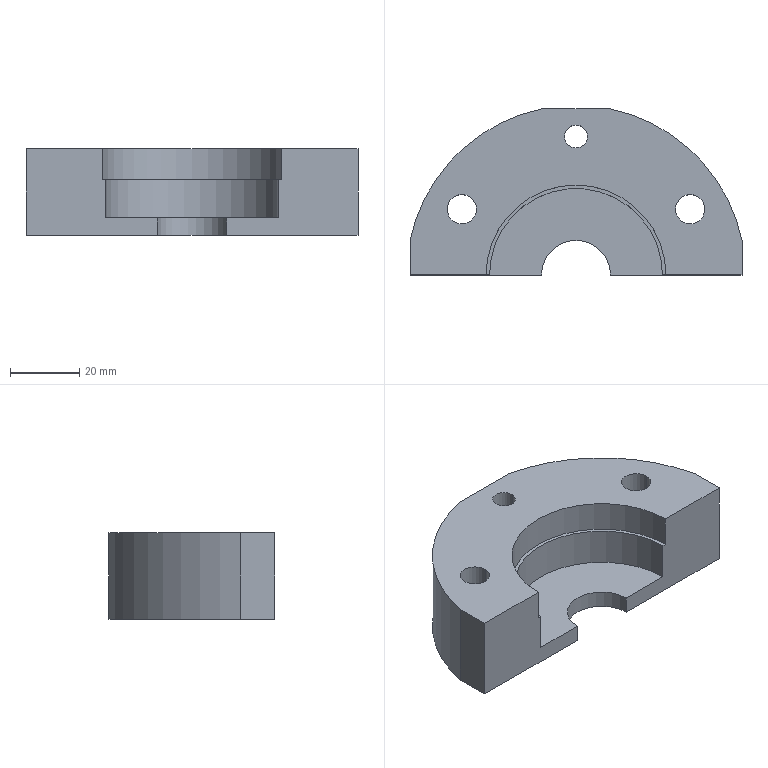Part | STEP file | 001-009-Riveting mechanism lower die floating block | 1 solid | 23 faces | box 96 x 48 x 25 mm | volume 68382 mm3 | cylinder 13 | plane 10 | commonest cylinder face diameters 8.5 x4 6.6 x2 11 x2 98 x2 20 x1 50 x1